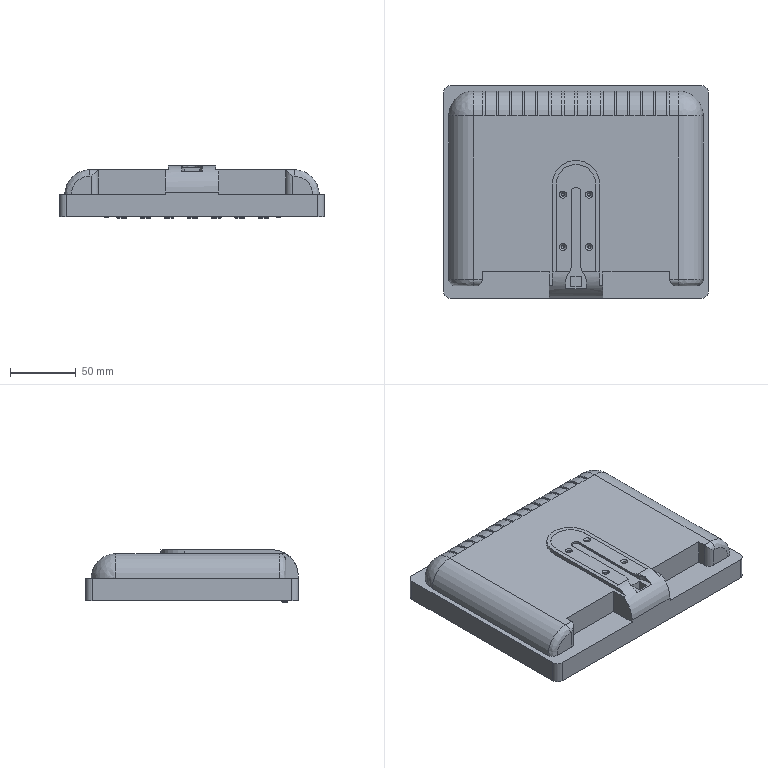Part | SolidWorks | features BaseBody 1 | 1 solid | 275 faces | box 202 x 162 x 40 mm | volume 1013492 mm3 | plane 119 | cylinder 103 | spline 29 | cone 24 | commonest cylinder face diameters 4.5 x21 38 x18 36.089 x15 1 x14 2.05 x8 2.9 x8